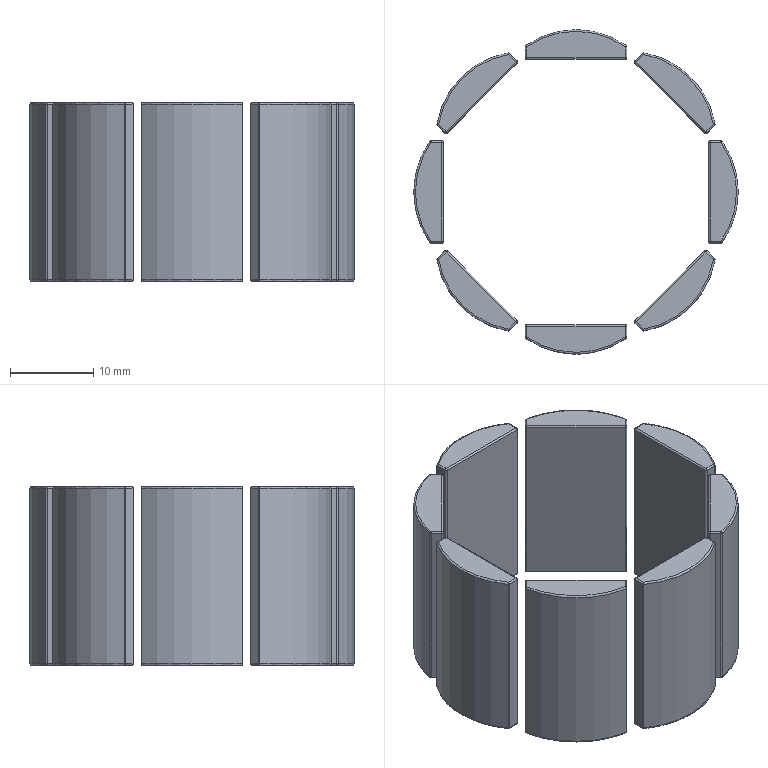Part | STEP file | TQ-DD-1105-THMagnet1010_デフォルト | 8 solids | 213 faces | box 39 x 39 x 21.5 mm | volume 6144 mm3 | cylinder 93 | spline 80 | plane 40 | commonest cylinder face diameters 0.4 x84 21 x9